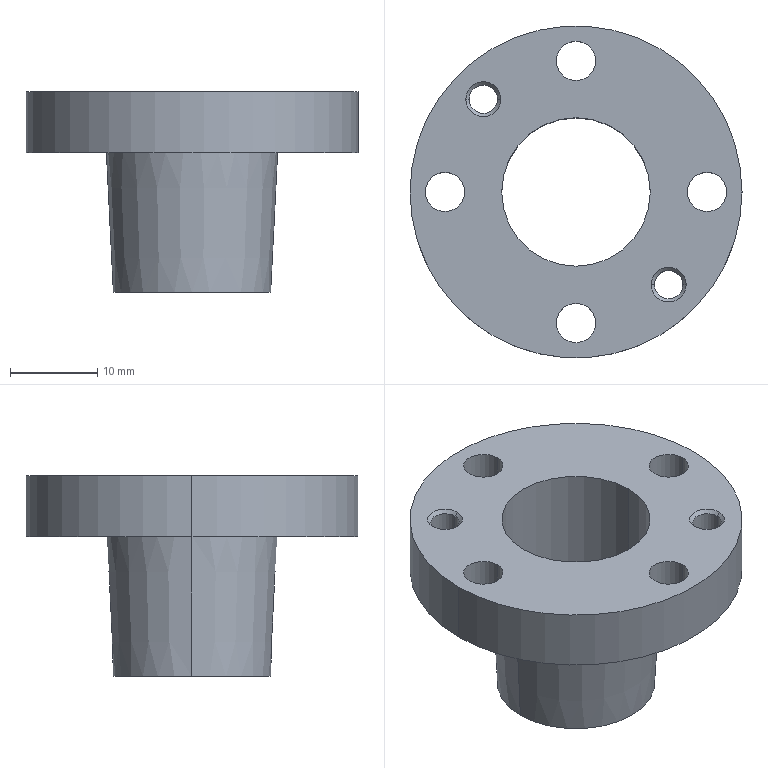Part | STEP file | LFSP35B_17_boltbushing | 1 solid | 29 faces | box 38 x 38 x 23 mm | volume 6598 mm3 | cylinder 16 | cone 10 | plane 3 | commonest cylinder face diameters 4.5 x8 3.242 x4 17 x2 38 x2